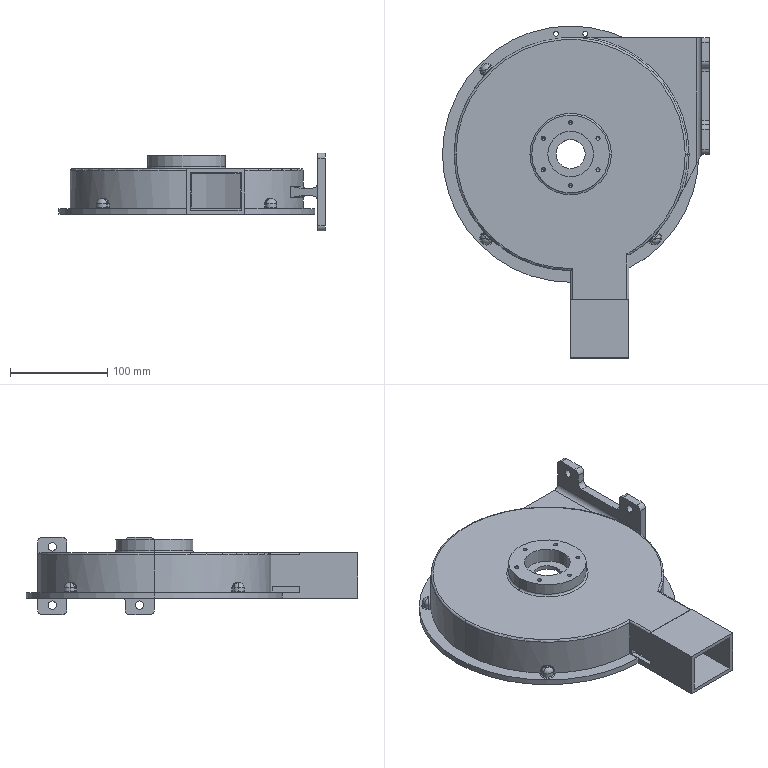Part | SolidWorks | features ICE 11, Fillet 10, BossThin 3, CirPattern 3, 3DProfileFeature 2, Cut 2, HoleWzd 2, Revolution 1 | 1 solid | 202 faces | box 275 x 342 x 80 mm | volume 622085 mm3 | cylinder 98 | plane 59 | torus 33 | cone 12 | commonest cylinder face diameters 10 x22 2 x18 4.2 x12 5 x12 8.5 x8 12 x6